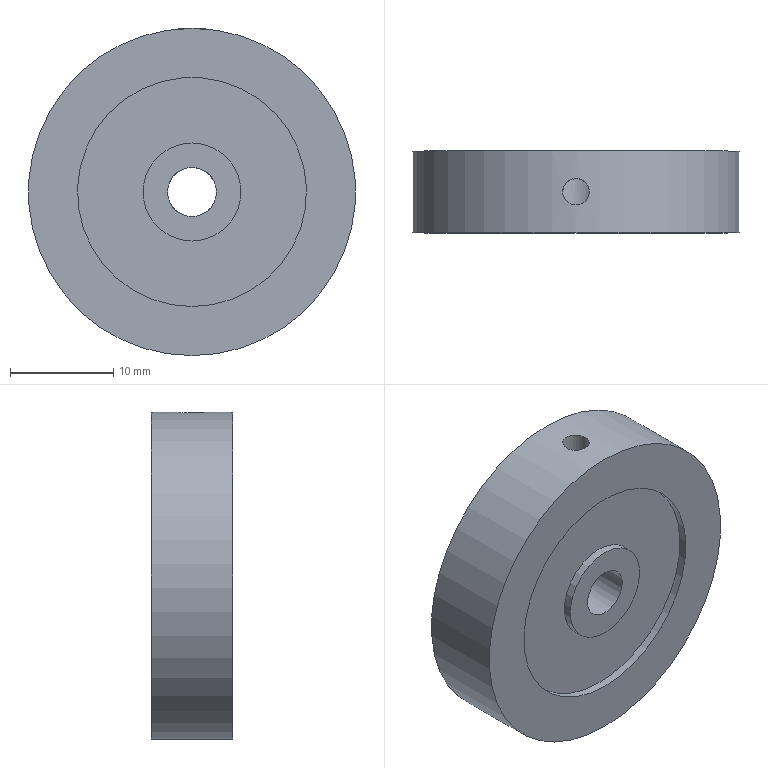Part | NX | features DATUM_CSYS 3, CYLINDER 2, SKETCH 2, DATUM_PLANE 1, SWP104 1 | 1 solid | 13 faces | box 31.75 x 7.938 x 31.75 mm | volume 5557 mm3 | cylinder 7 | plane 6 | commonest cylinder face diameters 9.525 x2 22.225 x2 2.578 x1 4.763 x1 31.75 x1
STEP:
#1=CARTESIAN_POINT('',(2.381,-3.969,0.));
#2=VERTEX_POINT('',#1);
#3=CARTESIAN_POINT('',(0.,-3.969,0.));
#4=DIRECTION('',(0.,1.,0.));
#5=DIRECTION('',(1.,0.,0.));
#6=AXIS2_PLACEMENT_3D('',#3,#4,#5);
#7=CIRCLE('',#6,2.381);
#8=EDGE_CURVE('',#2,#2,#7,.T.);
#9=ORIENTED_EDGE('',*,*,#8,.T.);
#10=EDGE_LOOP('',(#9));
#11=FACE_BOUND('',#10,.T.);
#12=CARTESIAN_POINT('',(0.,-3.969,-4.763));
#13=VERTEX_POINT('',#12);
#14=CARTESIAN_POINT('',(0.,-3.969,0.));
#15=DIRECTION('',(0.,-1.,0.));
#16=DIRECTION('',(0.,0.,-1.));
#17=AXIS2_PLACEMENT_3D('',#14,#15,#16);
#18=CIRCLE('',#17,4.763);
#19=EDGE_CURVE('',#13,#13,#18,.T.);
#20=ORIENTED_EDGE('',*,*,#19,.T.);
#21=EDGE_LOOP('',(#20));
#22=FACE_BOUND('',#21,.T.);
#23=CARTESIAN_POINT('',(0.,-3.969,4.763));
#24=DIRECTION('',(0.,1.,0.));
#25=DIRECTION('',(0.,0.,1.));
#26=AXIS2_PLACEMENT_3D('',#23,#24,#25);
#27=PLANE('',#26);
#28=ADVANCED_FACE('',(#11,#22),#27,.F.);
#29=CARTESIAN_POINT('',(0.,3.969,-2.381));
#30=VERTEX_POINT('',#29);
#31=CARTESIAN_POINT('',(0.,3.969,0.));
#32=DIRECTION('',(0.,-1.,0.));
#33=DIRECTION('',(0.,0.,-1.));
#34=AXIS2_PLACEMENT_3D('',#31,#32,#33);
#35=CIRCLE('',#34,2.381);
#36=EDGE_CURVE('',#30,#30,#35,.T.);
#37=ORIENTED_EDGE('',*,*,#36,.T.);
#38=EDGE_LOOP('',(#37));
#39=FACE_BOUND('',#38,.T.);
#40=CARTESIAN_POINT('',(0.,3.969,-4.763));
#41=VERTEX_POINT('',#40);
#42=CARTESIAN_POINT('',(0.,3.969,0.));
#43=DIRECTION('',(0.,-1.,0.));
#44=DIRECTION('',(0.,0.,-1.));
#45=AXIS2_PLACEMENT_3D('',#42,#43,#44);
#46=CIRCLE('',#45,4.763);
#47=EDGE_CURVE('',#41,#41,#46,.T.);
#48=ORIENTED_EDGE('',*,*,#47,.F.);
#49=EDGE_LOOP('',(#48));
#50=FACE_BOUND('',#49,.T.);
#51=CARTESIAN_POINT('',(0.,3.969,0.));
#52=DIRECTION('',(0.,-1.,0.));
#53=DIRECTION('',(0.,0.,-1.));
#54=AXIS2_PLACEMENT_3D('',#51,#52,#53);
#55=PLANE('',#54);
#56=ADVANCED_FACE('',(#39,#50),#55,.F.);
#57=CARTESIAN_POINT('',(0.,3.156,-4.763));
#58=VERTEX_POINT('',#57);
#59=CARTESIAN_POINT('',(0.,3.156,0.));
#60=DIRECTION('',(0.,-1.,0.));
#61=DIRECTION('',(0.,0.,-1.));
#62=AXIS2_PLACEMENT_3D('',#59,#60,#61);
#63=CIRCLE('',#62,4.763);
#64=EDGE_CURVE('',#58,#58,#63,.T.);
#65=ORIENTED_EDGE('',*,*,#64,.F.);
#66=EDGE_LOOP('',(#65));
#67=FACE_BOUND('',#66,.T.);
#68=ORIENTED_EDGE('',*,*,#47,.T.);
#69=EDGE_LOOP('',(#68));
#70=FACE_BOUND('',#69,.T.);
#71=CARTESIAN_POINT('',(0.,0.,0.));
#72=DIRECTION('',(0.,-1.,0.));
#73=DIRECTION('',(0.,0.,-1.));
#74=AXIS2_PLACEMENT_3D('',#71,#72,#73);
#75=CYLINDRICAL_SURFACE('',#74,4.763);
#76=ADVANCED_FACE('',(#67,#70),#75,.T.);
#77=CARTESIAN_POINT('',(0.,3.156,-11.113));
#78=VERTEX_POINT('',#77);
#79=CARTESIAN_POINT('',(0.,3.156,0.));
#80=DIRECTION('',(0.,-1.,0.));
#81=DIRECTION('',(0.,0.,-1.));
#82=AXIS2_PLACEMENT_3D('',#79,#80,#81);
#83=CIRCLE('',#82,11.113);
#84=EDGE_CURVE('',#78,#78,#83,.T.);
#85=ORIENTED_EDGE('',*,*,#84,.F.);
#86=EDGE_LOOP('',(#85));
#87=FACE_BOUND('',#86,.T.);
#88=ORIENTED_EDGE('',*,*,#64,.T.);
#89=EDGE_LOOP('',(#88));
#90=FACE_BOUND('',#89,.T.);
#91=CARTESIAN_POINT('',(0.,3.156,4.763));
#92=DIRECTION('',(0.,-1.,0.));
#93=DIRECTION('',(0.,0.,-1.));
#94=AXIS2_PLACEMENT_3D('',#91,#92,#93);
#95=PLANE('',#94);
#96=ADVANCED_FACE('',(#87,#90),#95,.F.);
#97=CARTESIAN_POINT('',(0.,3.969,-11.113));
#98=VERTEX_POINT('',#97);
#99=CARTESIAN_POINT('',(0.,3.969,0.));
#100=DIRECTION('',(0.,-1.,0.));
#101=DIRECTION('',(0.,0.,-1.));
#102=AXIS2_PLACEMENT_3D('',#99,#100,#101);
#103=CIRCLE('',#102,11.113);
#104=EDGE_CURVE('',#98,#98,#103,.T.);
#105=ORIENTED_EDGE('',*,*,#104,.F.);
#106=EDGE_LOOP('',(#105));
#107=FACE_BOUND('',#106,.T.);
#108=ORIENTED_EDGE('',*,*,#84,.T.);
#109=EDGE_LOOP('',(#108));
#110=FACE_BOUND('',#109,.T.);
#111=CARTESIAN_POINT('',(0.,0.,0.));
#112=DIRECTION('',(0.,-1.,0.));
#113=DIRECTION('',(0.,0.,-1.));
#114=AXIS2_PLACEMENT_3D('',#111,#112,#113);
#115=CYLINDRICAL_SURFACE('',#114,11.113);
#116=ADVANCED_FACE('',(#107,#110),#115,.F.);
#117=CARTESIAN_POINT('',(0.,3.969,-15.875));
#118=VERTEX_POINT('',#117);
#119=CARTESIAN_POINT('',(0.,3.969,0.));
#120=DIRECTION('',(0.,-1.,0.));
#121=DIRECTION('',(0.,0.,-1.));
#122=AXIS2_PLACEMENT_3D('',#119,#120,#121);
#123=CIRCLE('',#122,15.875);
#124=EDGE_CURVE('',#118,#118,#123,.T.);
#125=ORIENTED_EDGE('',*,*,#124,.F.);
#126=EDGE_LOOP('',(#125));
#127=FACE_BOUND('',#126,.T.);
#128=ORIENTED_EDGE('',*,*,#104,.T.);
#129=EDGE_LOOP('',(#128));
#130=FACE_BOUND('',#129,.T.);
#131=CARTESIAN_POINT('',(0.,3.969,11.113));
#132=DIRECTION('',(0.,-1.,0.));
#133=DIRECTION('',(0.,0.,-1.));
#134=AXIS2_PLACEMENT_3D('',#131,#132,#133);
#135=PLANE('',#134);
#136=ADVANCED_FACE('',(#127,#130),#135,.F.);
#137=CARTESIAN_POINT('',(0.,-1.289,15.875));
#138=VERTEX_POINT('',#137);
#139=CARTESIAN_POINT('',(1.011,-1.009,15.849));
#140=CARTESIAN_POINT('',(-0.0002554,-1.429,15.888));
#141=CARTESIAN_POINT('',(-1.01,-1.01,15.849));
#142=CARTESIAN_POINT('',(-1.428,-0.00109,15.809));
#143=CARTESIAN_POINT('',(-1.011,1.01,15.849));
#144=CARTESIAN_POINT('',(-0.0002287,1.428,15.888));
#145=CARTESIAN_POINT('',(1.009,1.011,15.849));
#146=CARTESIAN_POINT('',(1.429,0.001438,15.809));
#147=CARTESIAN_POINT('',(1.011,-1.009,15.849));
#148=CARTESIAN_POINT('',(-0.0002554,-1.429,15.888));
#149=CARTESIAN_POINT('',(-1.01,-1.01,15.849));
#150=B_SPLINE_CURVE_WITH_KNOTS('',3,(#139,#140,#141,#142,#143,#144,#145,#146,#147,#148,#149),.UNSPECIFIED.,.T.,.F.,(1,1,1,1,1,1,1,1,1,1,1,1,1,1,1),(-0.003024,-0.002016,-0.001008,0.,0.001008,0.002016,0.003024,0.004031,0.005039,0.006047,0.007055,0.008063,0.009071,0.01008,0.01109),.UNSPECIFIED.);
#151=EDGE_CURVE('',#138,#138,#150,.T.);
#152=ORIENTED_EDGE('',*,*,#151,.T.);
#153=EDGE_LOOP('',(#152));
#154=FACE_BOUND('',#153,.T.);
#155=CARTESIAN_POINT('',(0.,-3.969,-15.875));
#156=VERTEX_POINT('',#155);
#157=CARTESIAN_POINT('',(0.,-3.969,0.));
#158=DIRECTION('',(0.,-1.,0.));
#159=DIRECTION('',(0.,0.,-1.));
#160=AXIS2_PLACEMENT_3D('',#157,#158,#159);
#161=CIRCLE('',#160,15.875);
#162=EDGE_CURVE('',#156,#156,#161,.T.);
#163=ORIENTED_EDGE('',*,*,#162,.F.);
#164=EDGE_LOOP('',(#163));
#165=FACE_BOUND('',#164,.T.);
#166=ORIENTED_EDGE('',*,*,#124,.T.);
#167=EDGE_LOOP('',(#166));
#168=FACE_BOUND('',#167,.T.);
#169=CARTESIAN_POINT('',(0.,0.,0.));
#170=DIRECTION('',(0.,-1.,0.));
#171=DIRECTION('',(0.,0.,-1.));
#172=AXIS2_PLACEMENT_3D('',#169,#170,#171);
#173=CYLINDRICAL_SURFACE('',#172,15.875);
#174=ADVANCED_FACE('',(#154,#165,#168),#173,.T.);
#175=CARTESIAN_POINT('',(0.,-3.969,-11.113));
#176=VERTEX_POINT('',#175);
#177=CARTESIAN_POINT('',(0.,-3.969,0.));
#178=DIRECTION('',(0.,-1.,0.));
#179=DIRECTION('',(0.,0.,-1.));
#180=AXIS2_PLACEMENT_3D('',#177,#178,#179);
#181=CIRCLE('',#180,11.113);
#182=EDGE_CURVE('',#176,#176,#181,.T.);
#183=ORIENTED_EDGE('',*,*,#182,.F.);
#184=EDGE_LOOP('',(#183));
#185=FACE_BOUND('',#184,.T.);
#186=ORIENTED_EDGE('',*,*,#162,.T.);
#187=EDGE_LOOP('',(#186));
#188=FACE_BOUND('',#187,.T.);
#189=CARTESIAN_POINT('',(0.,-3.969,15.875));
#190=DIRECTION('',(0.,1.,0.));
#191=DIRECTION('',(0.,0.,1.));
#192=AXIS2_PLACEMENT_3D('',#189,#190,#191);
#193=PLANE('',#192);
#194=ADVANCED_FACE('',(#185,#188),#193,.F.);
#195=CARTESIAN_POINT('',(0.,-3.156,-11.113));
#196=VERTEX_POINT('',#195);
#197=CARTESIAN_POINT('',(0.,-3.156,0.));
#198=DIRECTION('',(0.,-1.,0.));
#199=DIRECTION('',(0.,0.,-1.));
#200=AXIS2_PLACEMENT_3D('',#197,#198,#199);
#201=CIRCLE('',#200,11.113);
#202=EDGE_CURVE('',#196,#196,#201,.T.);
#203=ORIENTED_EDGE('',*,*,#202,.F.);
#204=EDGE_LOOP('',(#203));
#205=FACE_BOUND('',#204,.T.);
#206=ORIENTED_EDGE('',*,*,#182,.T.);
#207=EDGE_LOOP('',(#206));
#208=FACE_BOUND('',#207,.T.);
#209=CARTESIAN_POINT('',(0.,0.,0.));
#210=DIRECTION('',(0.,-1.,0.));
#211=DIRECTION('',(0.,0.,-1.));
#212=AXIS2_PLACEMENT_3D('',#209,#210,#211);
#213=CYLINDRICAL_SURFACE('',#212,11.113);
#214=ADVANCED_FACE('',(#205,#208),#213,.F.);
#215=CARTESIAN_POINT('',(0.,-3.156,-4.763));
#216=VERTEX_POINT('',#215);
#217=CARTESIAN_POINT('',(0.,-3.156,0.));
#218=DIRECTION('',(0.,-1.,0.));
#219=DIRECTION('',(0.,0.,-1.));
#220=AXIS2_PLACEMENT_3D('',#217,#218,#219);
#221=CIRCLE('',#220,4.763);
#222=EDGE_CURVE('',#216,#216,#221,.T.);
#223=ORIENTED_EDGE('',*,*,#222,.F.);
#224=EDGE_LOOP('',(#223));
#225=FACE_BOUND('',#224,.T.);
#226=ORIENTED_EDGE('',*,*,#202,.T.);
#227=EDGE_LOOP('',(#226));
#228=FACE_BOUND('',#227,.T.);
#229=CARTESIAN_POINT('',(0.,-3.156,11.113));
#230=DIRECTION('',(0.,1.,0.));
#231=DIRECTION('',(0.,0.,1.));
#232=AXIS2_PLACEMENT_3D('',#229,#230,#231);
#233=PLANE('',#232);
#234=ADVANCED_FACE('',(#225,#228),#233,.F.);
#235=ORIENTED_EDGE('',*,*,#19,.F.);
#236=EDGE_LOOP('',(#235));
#237=FACE_BOUND('',#236,.T.);
#238=ORIENTED_EDGE('',*,*,#222,.T.);
#239=EDGE_LOOP('',(#238));
#240=FACE_BOUND('',#239,.T.);
#241=CARTESIAN_POINT('',(0.,0.,0.));
#242=DIRECTION('',(0.,-1.,0.));
#243=DIRECTION('',(0.,0.,-1.));
#244=AXIS2_PLACEMENT_3D('',#241,#242,#243);
#245=CYLINDRICAL_SURFACE('',#244,4.763);
#246=ADVANCED_FACE('',(#237,#240),#245,.T.);
#247=CARTESIAN_POINT('',(1.289,0.,2.002));
#248=VERTEX_POINT('',#247);
#249=CARTESIAN_POINT('',(1.012,-1.01,2.208));
#250=CARTESIAN_POINT('',(1.428,0.0006348,1.9));
#251=CARTESIAN_POINT('',(1.011,1.007,2.207));
#252=CARTESIAN_POINT('',(0.004973,1.429,2.468));
#253=CARTESIAN_POINT('',(-1.011,1.009,2.208));
#254=CARTESIAN_POINT('',(-1.428,0.006925,1.9));
#255=CARTESIAN_POINT('',(-1.013,-1.007,2.206));
#256=CARTESIAN_POINT('',(-0.005737,-1.429,2.468));
#257=CARTESIAN_POINT('',(1.012,-1.01,2.208));
#258=CARTESIAN_POINT('',(1.428,0.0006348,1.9));
#259=CARTESIAN_POINT('',(1.011,1.007,2.207));
#260=B_SPLINE_CURVE_WITH_KNOTS('',3,(#249,#250,#251,#252,#253,#254,#255,#256,#257,#258,#259),.UNSPECIFIED.,.T.,.F.,(1,1,1,1,1,1,1,1,1,1,1,1,1,1,1),(-0.003082,-0.002054,-0.001027,0.,0.001027,0.002054,0.003082,0.004109,0.005136,0.006163,0.00719,0.008217,0.009245,0.01027,0.0113),.UNSPECIFIED.);
#261=EDGE_CURVE('',#248,#248,#260,.T.);
#262=ORIENTED_EDGE('',*,*,#261,.T.);
#263=EDGE_LOOP('',(#262));
#264=FACE_BOUND('',#263,.T.);
#265=ORIENTED_EDGE('',*,*,#8,.F.);
#266=EDGE_LOOP('',(#265));
#267=FACE_BOUND('',#266,.T.);
#268=ORIENTED_EDGE('',*,*,#36,.F.);
#269=EDGE_LOOP('',(#268));
#270=FACE_BOUND('',#269,.T.);
#271=CARTESIAN_POINT('',(0.,-3.969,0.));
#272=DIRECTION('',(0.,1.,0.));
#273=DIRECTION('',(1.,0.,0.));
#274=AXIS2_PLACEMENT_3D('',#271,#272,#273);
#275=CYLINDRICAL_SURFACE('',#274,2.381);
#276=ADVANCED_FACE('',(#264,#267,#270),#275,.F.);
#277=ORIENTED_EDGE('',*,*,#261,.F.);
#278=EDGE_LOOP('',(#277));
#279=FACE_BOUND('',#278,.T.);
#280=ORIENTED_EDGE('',*,*,#151,.F.);
#281=EDGE_LOOP('',(#280));
#282=FACE_BOUND('',#281,.T.);
#283=CARTESIAN_POINT('',(0.,0.,15.875));
#284=DIRECTION('',(0.,0.,-1.));
#285=DIRECTION('',(1.,0.,0.));
#286=AXIS2_PLACEMENT_3D('',#283,#284,#285);
#287=CYLINDRICAL_SURFACE('',#286,1.289);
#288=ADVANCED_FACE('',(#279,#282),#287,.F.);
#289=CLOSED_SHELL('',(#28,#56,#76,#96,#116,#136,#174,#194,#214,#234,#246,#276,#288));
#290=MANIFOLD_SOLID_BREP('',#289);
#291=(LENGTH_UNIT()NAMED_UNIT(*)SI_UNIT(.MILLI.,.METRE.));
#292=UNCERTAINTY_MEASURE_WITH_UNIT(LENGTH_MEASURE(0.0508),#291,'','');
#293=(NAMED_UNIT(*)PLANE_ANGLE_UNIT()SI_UNIT($,.RADIAN.));
#294=(NAMED_UNIT(*)SI_UNIT($,.STERADIAN.)SOLID_ANGLE_UNIT());
#295=(GEOMETRIC_REPRESENTATION_CONTEXT(3)GLOBAL_UNCERTAINTY_ASSIGNED_CONTEXT((#292))GLOBAL_UNIT_ASSIGNED_CONTEXT((#291,#293,#294))REPRESENTATION_CONTEXT('',''));
#296=ADVANCED_BREP_SHAPE_REPRESENTATION('',(#290),#295);